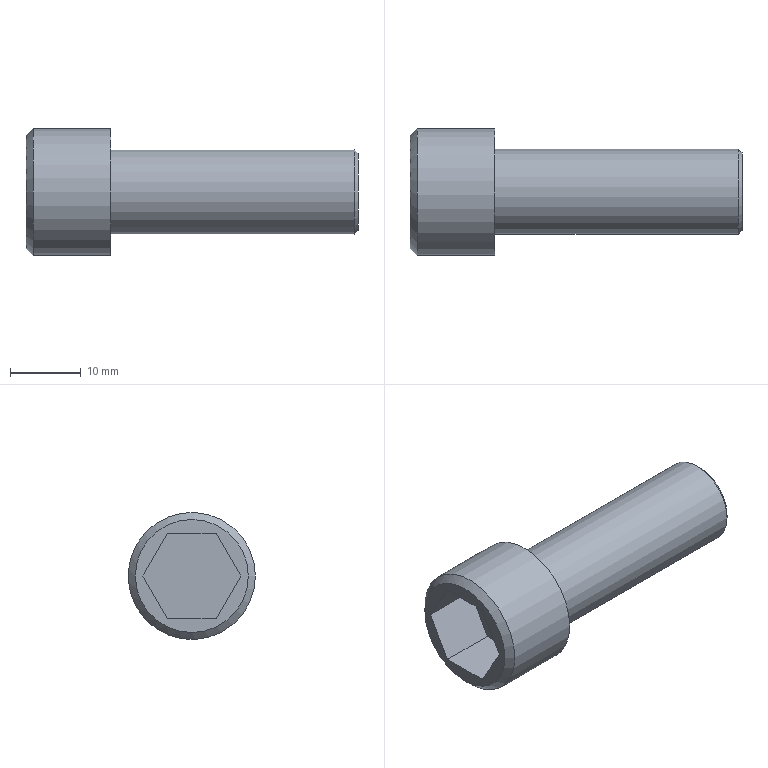Part | NX | features solid 2 | 1 solid | 14 faces | box 47 x 18 x 18 mm | volume 5983 mm3 | plane 10 | cylinder 2 | cone 2 | commonest cylinder face diameters 12 x1 18 x1
STEP:
#1=CARTESIAN_POINT('',(-54.,721.,-79.));
#2=VERTEX_POINT('',#1);
#3=CARTESIAN_POINT('',(-54.,730.,-79.));
#4=DIRECTION('',(-1.,0.,0.));
#5=DIRECTION('',(0.,-1.,0.));
#6=AXIS2_PLACEMENT_3D('',#3,#4,#5);
#7=CIRCLE('',#6,9.);
#8=EDGE_CURVE('',#2,#2,#7,.F.);
#9=ORIENTED_EDGE('',*,*,#8,.T.);
#10=EDGE_LOOP('',(#9));
#11=FACE_BOUND('',#10,.T.);
#12=CARTESIAN_POINT('',(-43.,721.,-79.));
#13=VERTEX_POINT('',#12);
#14=CARTESIAN_POINT('',(-43.,730.,-79.));
#15=DIRECTION('',(-1.,0.,0.));
#16=DIRECTION('',(0.,-1.,0.));
#17=AXIS2_PLACEMENT_3D('',#14,#15,#16);
#18=CIRCLE('',#17,9.);
#19=EDGE_CURVE('',#13,#13,#18,.T.);
#20=ORIENTED_EDGE('',*,*,#19,.T.);
#21=EDGE_LOOP('',(#20));
#22=FACE_BOUND('',#21,.T.);
#23=CARTESIAN_POINT('',(-43.,730.,-79.));
#24=DIRECTION('',(-1.,0.,0.));
#25=DIRECTION('',(0.,-1.,0.));
#26=AXIS2_PLACEMENT_3D('',#23,#24,#25);
#27=CYLINDRICAL_SURFACE('',#26,9.);
#28=ADVANCED_FACE('',(#11,#22),#27,.T.);
#29=CARTESIAN_POINT('',(-43.,736.,-79.));
#30=VERTEX_POINT('',#29);
#31=CARTESIAN_POINT('',(-43.,730.,-79.));
#32=DIRECTION('',(1.,0.,0.));
#33=DIRECTION('',(0.,1.,0.));
#34=AXIS2_PLACEMENT_3D('',#31,#32,#33);
#35=CIRCLE('',#34,6.);
#36=EDGE_CURVE('',#30,#30,#35,.T.);
#37=ORIENTED_EDGE('',*,*,#36,.F.);
#38=EDGE_LOOP('',(#37));
#39=FACE_BOUND('',#38,.T.);
#40=ORIENTED_EDGE('',*,*,#19,.F.);
#41=EDGE_LOOP('',(#40));
#42=FACE_BOUND('',#41,.T.);
#43=CARTESIAN_POINT('',(-43.,730.,-79.));
#44=DIRECTION('',(-1.,0.,0.));
#45=DIRECTION('',(0.,-1.,0.));
#46=AXIS2_PLACEMENT_3D('',#43,#44,#45);
#47=PLANE('',#46);
#48=ADVANCED_FACE('',(#39,#42),#47,.F.);
#49=CARTESIAN_POINT('',(-55.,722.,-79.));
#50=VERTEX_POINT('',#49);
#51=CARTESIAN_POINT('',(-55.,730.,-79.));
#52=DIRECTION('',(-1.,0.,0.));
#53=DIRECTION('',(0.,-1.,0.));
#54=AXIS2_PLACEMENT_3D('',#51,#52,#53);
#55=CIRCLE('',#54,8.);
#56=EDGE_CURVE('',#50,#50,#55,.T.);
#57=ORIENTED_EDGE('',*,*,#56,.T.);
#58=EDGE_LOOP('',(#57));
#59=FACE_BOUND('',#58,.T.);
#60=CARTESIAN_POINT('',(-55.,733.464,-73.));
#61=VERTEX_POINT('',#60);
#62=CARTESIAN_POINT('',(-55.,736.928,-79.));
#63=VERTEX_POINT('',#62);
#64=CARTESIAN_POINT('',(-55.,733.464,-73.));
#65=DIRECTION('',(0.,0.5,-0.866));
#66=VECTOR('',#65,1000.);
#67=LINE('',#64,#66);
#68=EDGE_CURVE('',#61,#63,#67,.T.);
#69=ORIENTED_EDGE('',*,*,#68,.F.);
#70=CARTESIAN_POINT('',(-55.,726.536,-73.));
#71=VERTEX_POINT('',#70);
#72=CARTESIAN_POINT('',(-55.,726.536,-73.));
#73=DIRECTION('',(0.,1.,0.));
#74=VECTOR('',#73,1000.);
#75=LINE('',#72,#74);
#76=EDGE_CURVE('',#71,#61,#75,.T.);
#77=ORIENTED_EDGE('',*,*,#76,.F.);
#78=CARTESIAN_POINT('',(-55.,723.072,-79.));
#79=VERTEX_POINT('',#78);
#80=CARTESIAN_POINT('',(-55.,723.072,-79.));
#81=DIRECTION('',(0.,0.5,0.866));
#82=VECTOR('',#81,1000.);
#83=LINE('',#80,#82);
#84=EDGE_CURVE('',#79,#71,#83,.T.);
#85=ORIENTED_EDGE('',*,*,#84,.F.);
#86=CARTESIAN_POINT('',(-55.,726.536,-85.));
#87=VERTEX_POINT('',#86);
#88=CARTESIAN_POINT('',(-55.,726.536,-85.));
#89=DIRECTION('',(0.,-0.5,0.866));
#90=VECTOR('',#89,1000.);
#91=LINE('',#88,#90);
#92=EDGE_CURVE('',#87,#79,#91,.T.);
#93=ORIENTED_EDGE('',*,*,#92,.F.);
#94=CARTESIAN_POINT('',(-55.,733.464,-85.));
#95=VERTEX_POINT('',#94);
#96=CARTESIAN_POINT('',(-55.,733.464,-85.));
#97=DIRECTION('',(0.,-1.,0.));
#98=VECTOR('',#97,1000.);
#99=LINE('',#96,#98);
#100=EDGE_CURVE('',#95,#87,#99,.T.);
#101=ORIENTED_EDGE('',*,*,#100,.F.);
#102=CARTESIAN_POINT('',(-55.,736.928,-79.));
#103=DIRECTION('',(0.,-0.5,-0.866));
#104=VECTOR('',#103,1000.);
#105=LINE('',#102,#104);
#106=EDGE_CURVE('',#63,#95,#105,.T.);
#107=ORIENTED_EDGE('',*,*,#106,.F.);
#108=EDGE_LOOP('',(#69,#77,#85,#93,#101,#107));
#109=FACE_BOUND('',#108,.T.);
#110=CARTESIAN_POINT('',(-55.,730.,-79.));
#111=DIRECTION('',(-1.,0.,0.));
#112=DIRECTION('',(0.,-1.,0.));
#113=AXIS2_PLACEMENT_3D('',#110,#111,#112);
#114=PLANE('',#113);
#115=ADVANCED_FACE('',(#59,#109),#114,.T.);
#116=CARTESIAN_POINT('',(-8.,735.5,-79.));
#117=VERTEX_POINT('',#116);
#118=CARTESIAN_POINT('',(-8.,730.,-79.));
#119=DIRECTION('',(1.,0.,0.));
#120=DIRECTION('',(0.,1.,0.));
#121=AXIS2_PLACEMENT_3D('',#118,#119,#120);
#122=CIRCLE('',#121,5.5);
#123=EDGE_CURVE('',#117,#117,#122,.T.);
#124=ORIENTED_EDGE('',*,*,#123,.T.);
#125=EDGE_LOOP('',(#124));
#126=FACE_BOUND('',#125,.T.);
#127=CARTESIAN_POINT('',(-8.,730.,-79.));
#128=DIRECTION('',(1.,0.,0.));
#129=DIRECTION('',(0.,1.,0.));
#130=AXIS2_PLACEMENT_3D('',#127,#128,#129);
#131=PLANE('',#130);
#132=ADVANCED_FACE('',(#126),#131,.T.);
#133=CARTESIAN_POINT('',(-8.5,736.,-79.));
#134=VERTEX_POINT('',#133);
#135=CARTESIAN_POINT('',(-8.5,730.,-79.));
#136=DIRECTION('',(1.,0.,0.));
#137=DIRECTION('',(0.,1.,0.));
#138=AXIS2_PLACEMENT_3D('',#135,#136,#137);
#139=CIRCLE('',#138,6.);
#140=EDGE_CURVE('',#134,#134,#139,.F.);
#141=ORIENTED_EDGE('',*,*,#140,.T.);
#142=EDGE_LOOP('',(#141));
#143=FACE_BOUND('',#142,.T.);
#144=ORIENTED_EDGE('',*,*,#36,.T.);
#145=EDGE_LOOP('',(#144));
#146=FACE_BOUND('',#145,.T.);
#147=CARTESIAN_POINT('',(-43.,730.,-79.));
#148=DIRECTION('',(1.,0.,0.));
#149=DIRECTION('',(0.,1.,0.));
#150=AXIS2_PLACEMENT_3D('',#147,#148,#149);
#151=CYLINDRICAL_SURFACE('',#150,6.);
#152=ADVANCED_FACE('',(#143,#146),#151,.T.);
#153=ORIENTED_EDGE('',*,*,#68,.T.);
#154=CARTESIAN_POINT('',(-47.,736.928,-79.));
#155=VERTEX_POINT('',#154);
#156=CARTESIAN_POINT('',(-47.,736.928,-79.));
#157=DIRECTION('',(-1.,0.,0.));
#158=VECTOR('',#157,1000.);
#159=LINE('',#156,#158);
#160=EDGE_CURVE('',#155,#63,#159,.T.);
#161=ORIENTED_EDGE('',*,*,#160,.F.);
#162=CARTESIAN_POINT('',(-47.,733.464,-73.));
#163=VERTEX_POINT('',#162);
#164=CARTESIAN_POINT('',(-47.,733.464,-73.));
#165=DIRECTION('',(0.,0.5,-0.866));
#166=VECTOR('',#165,1000.);
#167=LINE('',#164,#166);
#168=EDGE_CURVE('',#163,#155,#167,.T.);
#169=ORIENTED_EDGE('',*,*,#168,.F.);
#170=CARTESIAN_POINT('',(-47.,733.464,-73.));
#171=DIRECTION('',(-1.,0.,0.));
#172=VECTOR('',#171,1000.);
#173=LINE('',#170,#172);
#174=EDGE_CURVE('',#163,#61,#173,.T.);
#175=ORIENTED_EDGE('',*,*,#174,.T.);
#176=EDGE_LOOP('',(#153,#161,#169,#175));
#177=FACE_BOUND('',#176,.T.);
#178=CARTESIAN_POINT('',(-47.,733.464,-73.));
#179=DIRECTION('',(0.,0.866,0.5));
#180=DIRECTION('',(0.,0.5,-0.866));
#181=AXIS2_PLACEMENT_3D('',#178,#179,#180);
#182=PLANE('',#181);
#183=ADVANCED_FACE('',(#177),#182,.F.);
#184=ORIENTED_EDGE('',*,*,#106,.T.);
#185=CARTESIAN_POINT('',(-47.,733.464,-85.));
#186=VERTEX_POINT('',#185);
#187=CARTESIAN_POINT('',(-47.,733.464,-85.));
#188=DIRECTION('',(-1.,0.,0.));
#189=VECTOR('',#188,1000.);
#190=LINE('',#187,#189);
#191=EDGE_CURVE('',#186,#95,#190,.T.);
#192=ORIENTED_EDGE('',*,*,#191,.F.);
#193=CARTESIAN_POINT('',(-47.,736.928,-79.));
#194=DIRECTION('',(0.,-0.5,-0.866));
#195=VECTOR('',#194,1000.);
#196=LINE('',#193,#195);
#197=EDGE_CURVE('',#155,#186,#196,.T.);
#198=ORIENTED_EDGE('',*,*,#197,.F.);
#199=ORIENTED_EDGE('',*,*,#160,.T.);
#200=EDGE_LOOP('',(#184,#192,#198,#199));
#201=FACE_BOUND('',#200,.T.);
#202=CARTESIAN_POINT('',(-47.,736.928,-79.));
#203=DIRECTION('',(0.,0.866,-0.5));
#204=DIRECTION('',(0.,-0.5,-0.866));
#205=AXIS2_PLACEMENT_3D('',#202,#203,#204);
#206=PLANE('',#205);
#207=ADVANCED_FACE('',(#201),#206,.F.);
#208=ORIENTED_EDGE('',*,*,#100,.T.);
#209=CARTESIAN_POINT('',(-47.,726.536,-85.));
#210=VERTEX_POINT('',#209);
#211=CARTESIAN_POINT('',(-47.,726.536,-85.));
#212=DIRECTION('',(-1.,0.,0.));
#213=VECTOR('',#212,1000.);
#214=LINE('',#211,#213);
#215=EDGE_CURVE('',#210,#87,#214,.T.);
#216=ORIENTED_EDGE('',*,*,#215,.F.);
#217=CARTESIAN_POINT('',(-47.,733.464,-85.));
#218=DIRECTION('',(0.,-1.,0.));
#219=VECTOR('',#218,1000.);
#220=LINE('',#217,#219);
#221=EDGE_CURVE('',#186,#210,#220,.T.);
#222=ORIENTED_EDGE('',*,*,#221,.F.);
#223=ORIENTED_EDGE('',*,*,#191,.T.);
#224=EDGE_LOOP('',(#208,#216,#222,#223));
#225=FACE_BOUND('',#224,.T.);
#226=CARTESIAN_POINT('',(-47.,733.464,-85.));
#227=DIRECTION('',(0.,0.,-1.));
#228=DIRECTION('',(1.,0.,0.));
#229=AXIS2_PLACEMENT_3D('',#226,#227,#228);
#230=PLANE('',#229);
#231=ADVANCED_FACE('',(#225),#230,.F.);
#232=ORIENTED_EDGE('',*,*,#92,.T.);
#233=CARTESIAN_POINT('',(-47.,723.072,-79.));
#234=VERTEX_POINT('',#233);
#235=CARTESIAN_POINT('',(-47.,723.072,-79.));
#236=DIRECTION('',(-1.,0.,0.));
#237=VECTOR('',#236,1000.);
#238=LINE('',#235,#237);
#239=EDGE_CURVE('',#234,#79,#238,.T.);
#240=ORIENTED_EDGE('',*,*,#239,.F.);
#241=CARTESIAN_POINT('',(-47.,726.536,-85.));
#242=DIRECTION('',(0.,-0.5,0.866));
#243=VECTOR('',#242,1000.);
#244=LINE('',#241,#243);
#245=EDGE_CURVE('',#210,#234,#244,.T.);
#246=ORIENTED_EDGE('',*,*,#245,.F.);
#247=ORIENTED_EDGE('',*,*,#215,.T.);
#248=EDGE_LOOP('',(#232,#240,#246,#247));
#249=FACE_BOUND('',#248,.T.);
#250=CARTESIAN_POINT('',(-47.,726.536,-85.));
#251=DIRECTION('',(0.,-0.866,-0.5));
#252=DIRECTION('',(0.,-0.5,0.866));
#253=AXIS2_PLACEMENT_3D('',#250,#251,#252);
#254=PLANE('',#253);
#255=ADVANCED_FACE('',(#249),#254,.F.);
#256=ORIENTED_EDGE('',*,*,#84,.T.);
#257=CARTESIAN_POINT('',(-47.,726.536,-73.));
#258=VERTEX_POINT('',#257);
#259=CARTESIAN_POINT('',(-47.,726.536,-73.));
#260=DIRECTION('',(-1.,0.,0.));
#261=VECTOR('',#260,1000.);
#262=LINE('',#259,#261);
#263=EDGE_CURVE('',#258,#71,#262,.T.);
#264=ORIENTED_EDGE('',*,*,#263,.F.);
#265=CARTESIAN_POINT('',(-47.,723.072,-79.));
#266=DIRECTION('',(0.,0.5,0.866));
#267=VECTOR('',#266,1000.);
#268=LINE('',#265,#267);
#269=EDGE_CURVE('',#234,#258,#268,.T.);
#270=ORIENTED_EDGE('',*,*,#269,.F.);
#271=ORIENTED_EDGE('',*,*,#239,.T.);
#272=EDGE_LOOP('',(#256,#264,#270,#271));
#273=FACE_BOUND('',#272,.T.);
#274=CARTESIAN_POINT('',(-47.,723.072,-79.));
#275=DIRECTION('',(0.,-0.866,0.5));
#276=DIRECTION('',(0.,0.5,0.866));
#277=AXIS2_PLACEMENT_3D('',#274,#275,#276);
#278=PLANE('',#277);
#279=ADVANCED_FACE('',(#273),#278,.F.);
#280=ORIENTED_EDGE('',*,*,#76,.T.);
#281=ORIENTED_EDGE('',*,*,#174,.F.);
#282=CARTESIAN_POINT('',(-47.,726.536,-73.));
#283=DIRECTION('',(0.,1.,0.));
#284=VECTOR('',#283,1000.);
#285=LINE('',#282,#284);
#286=EDGE_CURVE('',#258,#163,#285,.T.);
#287=ORIENTED_EDGE('',*,*,#286,.F.);
#288=ORIENTED_EDGE('',*,*,#263,.T.);
#289=EDGE_LOOP('',(#280,#281,#287,#288));
#290=FACE_BOUND('',#289,.T.);
#291=CARTESIAN_POINT('',(-47.,726.536,-73.));
#292=DIRECTION('',(0.,0.,1.));
#293=DIRECTION('',(0.,1.,0.));
#294=AXIS2_PLACEMENT_3D('',#291,#292,#293);
#295=PLANE('',#294);
#296=ADVANCED_FACE('',(#290),#295,.F.);
#297=ORIENTED_EDGE('',*,*,#168,.T.);
#298=ORIENTED_EDGE('',*,*,#197,.T.);
#299=ORIENTED_EDGE('',*,*,#221,.T.);
#300=ORIENTED_EDGE('',*,*,#245,.T.);
#301=ORIENTED_EDGE('',*,*,#269,.T.);
#302=ORIENTED_EDGE('',*,*,#286,.T.);
#303=EDGE_LOOP('',(#297,#298,#299,#300,#301,#302));
#304=FACE_BOUND('',#303,.T.);
#305=CARTESIAN_POINT('',(-47.,736.928,-79.));
#306=DIRECTION('',(-1.,0.,0.));
#307=DIRECTION('',(0.,-1.,0.));
#308=AXIS2_PLACEMENT_3D('',#305,#306,#307);
#309=PLANE('',#308);
#310=ADVANCED_FACE('',(#304),#309,.T.);
#311=ORIENTED_EDGE('',*,*,#8,.F.);
#312=EDGE_LOOP('',(#311));
#313=FACE_BOUND('',#312,.T.);
#314=ORIENTED_EDGE('',*,*,#56,.F.);
#315=EDGE_LOOP('',(#314));
#316=FACE_BOUND('',#315,.T.);
#317=CARTESIAN_POINT('',(-55.,730.,-79.));
#318=DIRECTION('',(1.,0.,0.));
#319=DIRECTION('',(0.,1.,0.));
#320=AXIS2_PLACEMENT_3D('',#317,#318,#319);
#321=CONICAL_SURFACE('',#320,8.,0.7854);
#322=ADVANCED_FACE('',(#313,#316),#321,.T.);
#323=ORIENTED_EDGE('',*,*,#140,.F.);
#324=EDGE_LOOP('',(#323));
#325=FACE_BOUND('',#324,.T.);
#326=ORIENTED_EDGE('',*,*,#123,.F.);
#327=EDGE_LOOP('',(#326));
#328=FACE_BOUND('',#327,.T.);
#329=CARTESIAN_POINT('',(-8.,730.,-79.));
#330=DIRECTION('',(-1.,0.,0.));
#331=DIRECTION('',(0.,-1.,0.));
#332=AXIS2_PLACEMENT_3D('',#329,#330,#331);
#333=CONICAL_SURFACE('',#332,5.5,0.7854);
#334=ADVANCED_FACE('',(#325,#328),#333,.T.);
#335=CLOSED_SHELL('',(#28,#48,#115,#132,#152,#183,#207,#231,#255,#279,#296,#310,#322,#334));
#336=MANIFOLD_SOLID_BREP('',#335);
#337=(LENGTH_UNIT()NAMED_UNIT(*)SI_UNIT(.MILLI.,.METRE.));
#338=UNCERTAINTY_MEASURE_WITH_UNIT(LENGTH_MEASURE(0.00001),#337,'','');
#339=(NAMED_UNIT(*)PLANE_ANGLE_UNIT()SI_UNIT($,.RADIAN.));
#340=(NAMED_UNIT(*)SI_UNIT($,.STERADIAN.)SOLID_ANGLE_UNIT());
#341=(GEOMETRIC_REPRESENTATION_CONTEXT(3)GLOBAL_UNCERTAINTY_ASSIGNED_CONTEXT((#338))GLOBAL_UNIT_ASSIGNED_CONTEXT((#337,#339,#340))REPRESENTATION_CONTEXT('',''));
#342=ADVANCED_BREP_SHAPE_REPRESENTATION('',(#336),#341);